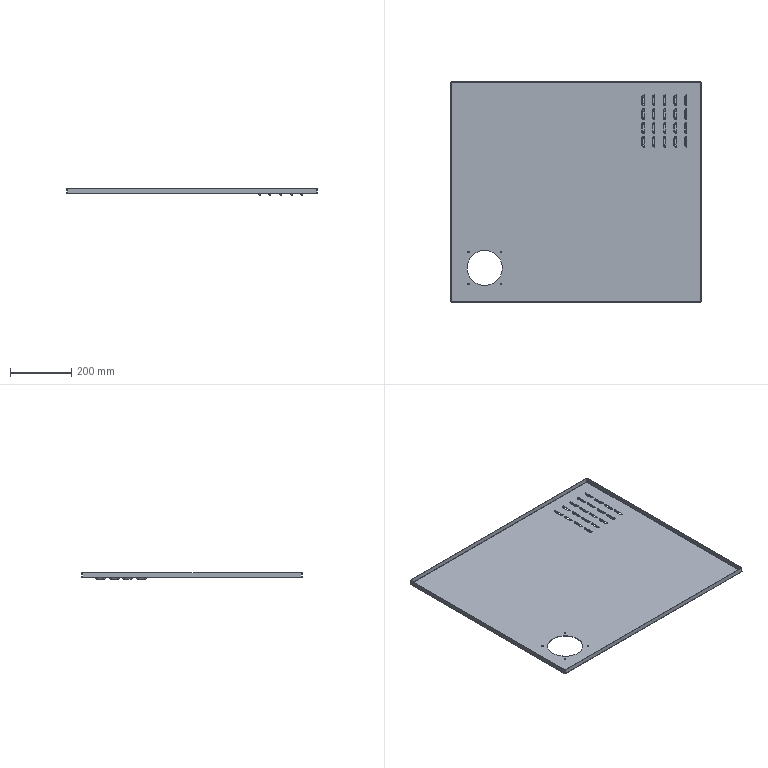Part | STEP file | Mirrored side cover plate1_mirror | 1 solid | 328 faces | box 818 x 718 x 22.2 mm | volume 748491 mm3 | cylinder 98 | torus 80 | sphere 80 | plane 62 | spline 8 | commonest cylinder face diameters 1.6 x20 4 x20 12 x20 14.4 x20 5 x8 0.4 x4